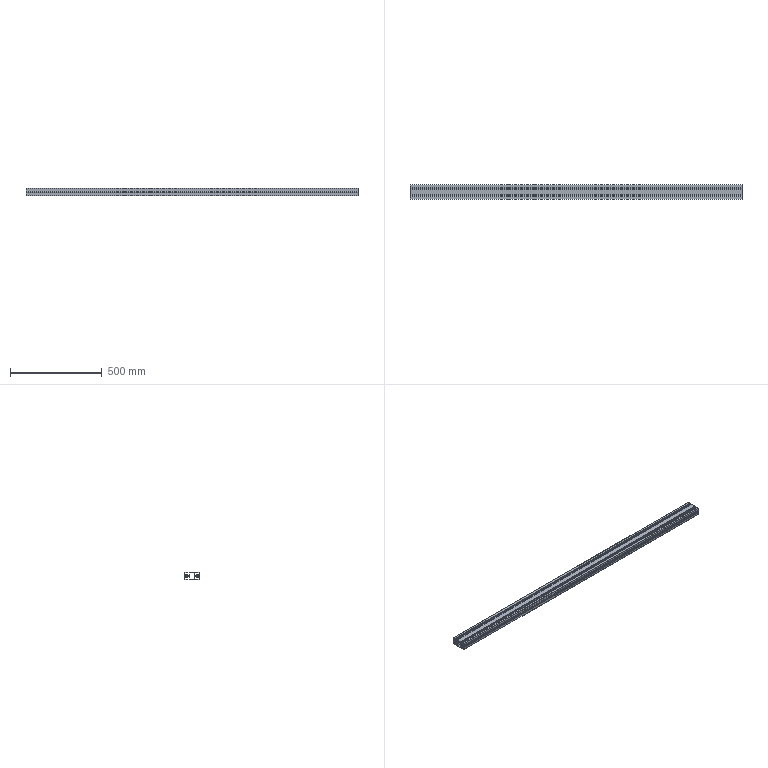Part | STEP file | Aluminium profile frame_Default<Machined> | 1 solid | 124 faces | box 1808 x 80 x 40 mm | volume 1339853 mm3 | plane 110 | cylinder 14 | commonest cylinder face diameters 9.6 x9 0.6 x2 6.6 x2 13.3 x1